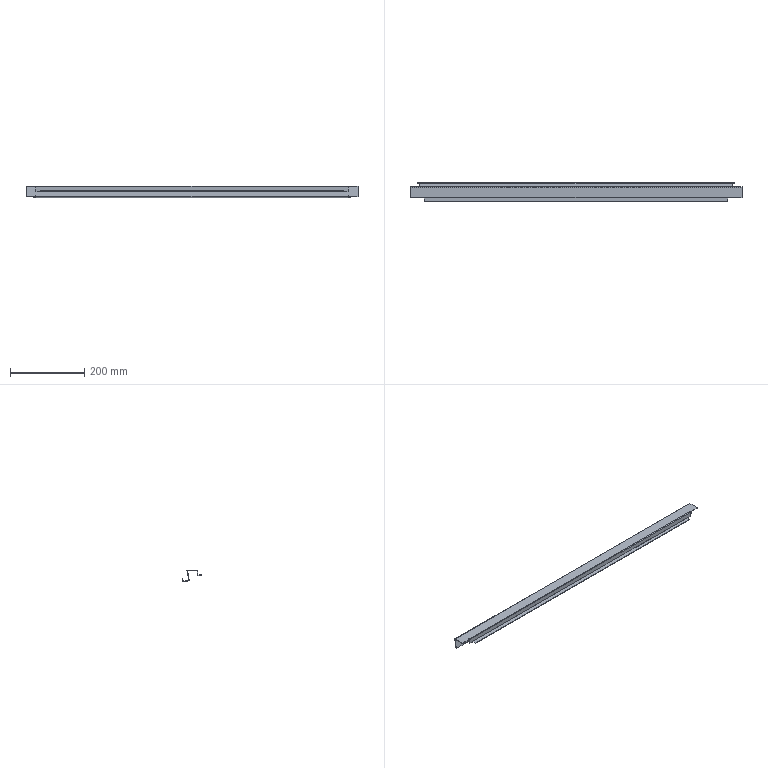Part | SolidWorks | features EdgeFlange 5, SMBaseFlange 2, FlatPattern 1, SheetMetal 1 | 1 solid | 78 faces | box 897 x 52.929 x 32.409 mm | volume 134963 mm3 | plane 68 | cylinder 10 | commonest cylinder face diameters 0.2 x5 3.2 x5